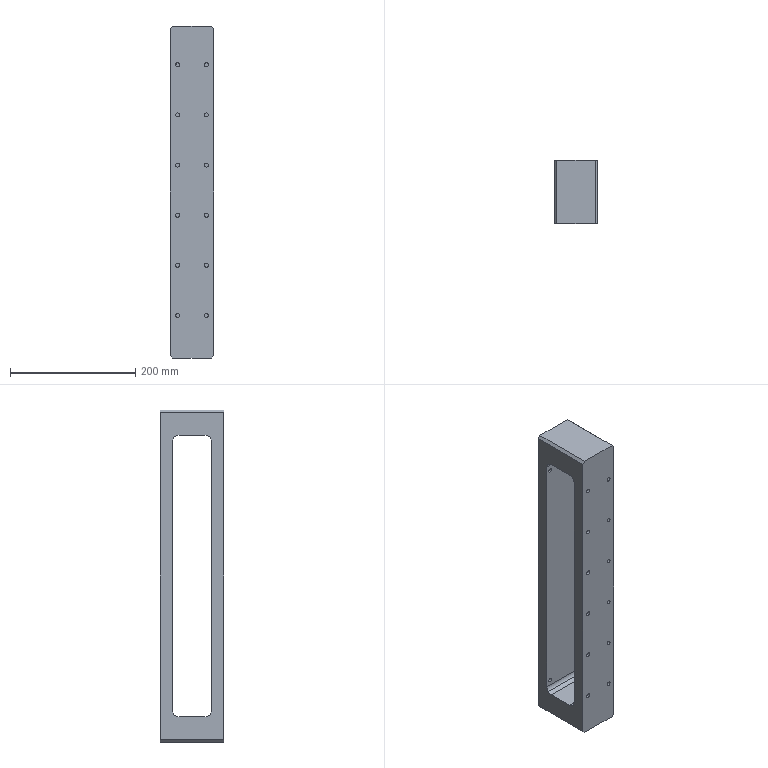Part | STEP file | ASND-0110-TCTF01-29 | 1 solid | 90 faces | box 70 x 101.1 x 530 mm | volume 1817903 mm3 | cylinder 56 | cone 20 | plane 14 | commonest cylinder face diameters 6.5 x24 4 x20 20 x8 6 x4